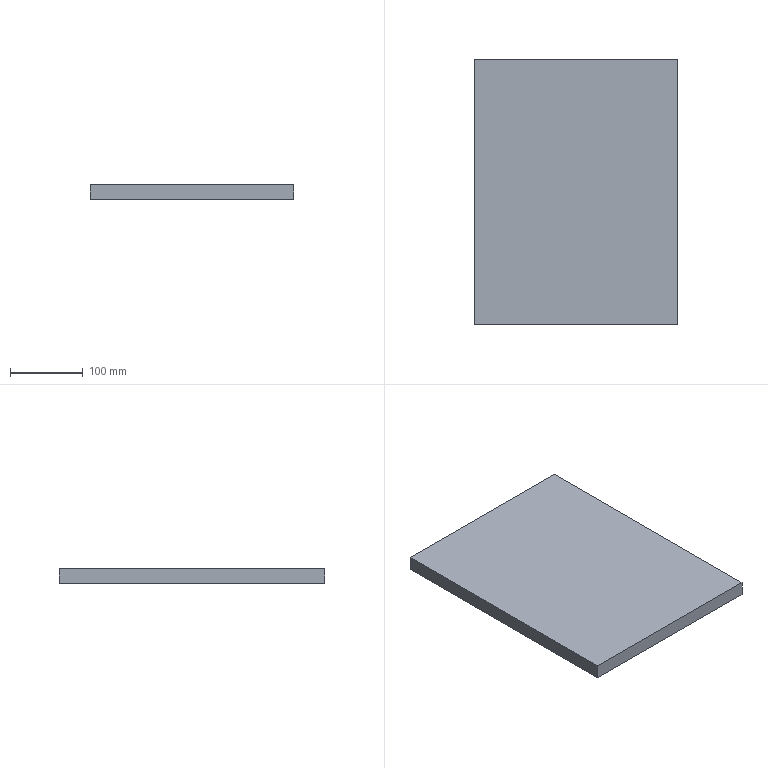Part | SolidWorks | features Extrusion 1 | 1 solid | 6 faces | box 280 x 365 x 20 mm | volume 2044000 mm3 | plane 6
STEP:
#1=CARTESIAN_POINT('',(0.,0.,0.));
#2=VERTEX_POINT('',#1);
#3=CARTESIAN_POINT('',(0.,365.,0.));
#4=VERTEX_POINT('',#3);
#5=CARTESIAN_POINT('',(0.,0.,0.));
#6=DIRECTION('',(0.,1.,0.));
#7=VECTOR('',#6,1000.);
#8=LINE('',#5,#7);
#9=EDGE_CURVE('',#2,#4,#8,.T.);
#10=ORIENTED_EDGE('',*,*,#9,.T.);
#11=CARTESIAN_POINT('',(0.,365.,20.));
#12=VERTEX_POINT('',#11);
#13=CARTESIAN_POINT('',(0.,365.,20.));
#14=DIRECTION('',(0.,0.,-1.));
#15=VECTOR('',#14,1000.);
#16=LINE('',#13,#15);
#17=EDGE_CURVE('',#12,#4,#16,.T.);
#18=ORIENTED_EDGE('',*,*,#17,.F.);
#19=CARTESIAN_POINT('',(0.,0.,20.));
#20=VERTEX_POINT('',#19);
#21=CARTESIAN_POINT('',(0.,0.,20.));
#22=DIRECTION('',(0.,1.,0.));
#23=VECTOR('',#22,1000.);
#24=LINE('',#21,#23);
#25=EDGE_CURVE('',#20,#12,#24,.T.);
#26=ORIENTED_EDGE('',*,*,#25,.F.);
#27=CARTESIAN_POINT('',(0.,0.,20.));
#28=DIRECTION('',(0.,0.,-1.));
#29=VECTOR('',#28,1000.);
#30=LINE('',#27,#29);
#31=EDGE_CURVE('',#20,#2,#30,.T.);
#32=ORIENTED_EDGE('',*,*,#31,.T.);
#33=EDGE_LOOP('',(#10,#18,#26,#32));
#34=FACE_OUTER_BOUND('',#33,.T.);
#35=CARTESIAN_POINT('',(0.,0.,20.));
#36=DIRECTION('',(-1.,0.,0.));
#37=DIRECTION('',(0.,0.,1.));
#38=AXIS2_PLACEMENT_3D('',#35,#36,#37);
#39=PLANE('',#38);
#40=ADVANCED_FACE('',(#34),#39,.F.);
#41=CARTESIAN_POINT('',(-280.,365.,0.));
#42=VERTEX_POINT('',#41);
#43=CARTESIAN_POINT('',(0.,365.,0.));
#44=DIRECTION('',(-1.,0.,0.));
#45=VECTOR('',#44,1000.);
#46=LINE('',#43,#45);
#47=EDGE_CURVE('',#4,#42,#46,.T.);
#48=ORIENTED_EDGE('',*,*,#47,.T.);
#49=CARTESIAN_POINT('',(-280.,365.,20.));
#50=VERTEX_POINT('',#49);
#51=CARTESIAN_POINT('',(-280.,365.,20.));
#52=DIRECTION('',(0.,0.,-1.));
#53=VECTOR('',#52,1000.);
#54=LINE('',#51,#53);
#55=EDGE_CURVE('',#50,#42,#54,.T.);
#56=ORIENTED_EDGE('',*,*,#55,.F.);
#57=CARTESIAN_POINT('',(0.,365.,20.));
#58=DIRECTION('',(-1.,0.,0.));
#59=VECTOR('',#58,1000.);
#60=LINE('',#57,#59);
#61=EDGE_CURVE('',#12,#50,#60,.T.);
#62=ORIENTED_EDGE('',*,*,#61,.F.);
#63=ORIENTED_EDGE('',*,*,#17,.T.);
#64=EDGE_LOOP('',(#48,#56,#62,#63));
#65=FACE_OUTER_BOUND('',#64,.T.);
#66=CARTESIAN_POINT('',(0.,365.,20.));
#67=DIRECTION('',(0.,-1.,0.));
#68=DIRECTION('',(1.,0.,0.));
#69=AXIS2_PLACEMENT_3D('',#66,#67,#68);
#70=PLANE('',#69);
#71=ADVANCED_FACE('',(#65),#70,.F.);
#72=CARTESIAN_POINT('',(-280.,0.,0.));
#73=VERTEX_POINT('',#72);
#74=CARTESIAN_POINT('',(-280.,0.,0.));
#75=DIRECTION('',(0.,-1.,0.));
#76=VECTOR('',#75,1000.);
#77=LINE('',#74,#76);
#78=EDGE_CURVE('',#42,#73,#77,.T.);
#79=ORIENTED_EDGE('',*,*,#78,.T.);
#80=CARTESIAN_POINT('',(-280.,0.,20.));
#81=VERTEX_POINT('',#80);
#82=CARTESIAN_POINT('',(-280.,0.,20.));
#83=DIRECTION('',(0.,0.,-1.));
#84=VECTOR('',#83,1000.);
#85=LINE('',#82,#84);
#86=EDGE_CURVE('',#81,#73,#85,.T.);
#87=ORIENTED_EDGE('',*,*,#86,.F.);
#88=CARTESIAN_POINT('',(-280.,0.,20.));
#89=DIRECTION('',(0.,-1.,0.));
#90=VECTOR('',#89,1000.);
#91=LINE('',#88,#90);
#92=EDGE_CURVE('',#50,#81,#91,.T.);
#93=ORIENTED_EDGE('',*,*,#92,.F.);
#94=ORIENTED_EDGE('',*,*,#55,.T.);
#95=EDGE_LOOP('',(#79,#87,#93,#94));
#96=FACE_OUTER_BOUND('',#95,.T.);
#97=CARTESIAN_POINT('',(-280.,0.,20.));
#98=DIRECTION('',(1.,0.,0.));
#99=DIRECTION('',(0.,0.,-1.));
#100=AXIS2_PLACEMENT_3D('',#97,#98,#99);
#101=PLANE('',#100);
#102=ADVANCED_FACE('',(#96),#101,.F.);
#103=CARTESIAN_POINT('',(0.,0.,0.));
#104=DIRECTION('',(1.,0.,0.));
#105=VECTOR('',#104,1000.);
#106=LINE('',#103,#105);
#107=EDGE_CURVE('',#73,#2,#106,.T.);
#108=ORIENTED_EDGE('',*,*,#107,.T.);
#109=ORIENTED_EDGE('',*,*,#31,.F.);
#110=CARTESIAN_POINT('',(0.,0.,20.));
#111=DIRECTION('',(1.,0.,0.));
#112=VECTOR('',#111,1000.);
#113=LINE('',#110,#112);
#114=EDGE_CURVE('',#81,#20,#113,.T.);
#115=ORIENTED_EDGE('',*,*,#114,.F.);
#116=ORIENTED_EDGE('',*,*,#86,.T.);
#117=EDGE_LOOP('',(#108,#109,#115,#116));
#118=FACE_OUTER_BOUND('',#117,.T.);
#119=CARTESIAN_POINT('',(0.,0.,20.));
#120=DIRECTION('',(0.,1.,0.));
#121=DIRECTION('',(-1.,0.,0.));
#122=AXIS2_PLACEMENT_3D('',#119,#120,#121);
#123=PLANE('',#122);
#124=ADVANCED_FACE('',(#118),#123,.F.);
#125=ORIENTED_EDGE('',*,*,#25,.T.);
#126=ORIENTED_EDGE('',*,*,#61,.T.);
#127=ORIENTED_EDGE('',*,*,#92,.T.);
#128=ORIENTED_EDGE('',*,*,#114,.T.);
#129=EDGE_LOOP('',(#125,#126,#127,#128));
#130=FACE_OUTER_BOUND('',#129,.T.);
#131=CARTESIAN_POINT('',(0.,0.,20.));
#132=DIRECTION('',(0.,0.,1.));
#133=DIRECTION('',(1.,0.,0.));
#134=AXIS2_PLACEMENT_3D('',#131,#132,#133);
#135=PLANE('',#134);
#136=ADVANCED_FACE('',(#130),#135,.T.);
#137=ORIENTED_EDGE('',*,*,#9,.F.);
#138=ORIENTED_EDGE('',*,*,#107,.F.);
#139=ORIENTED_EDGE('',*,*,#78,.F.);
#140=ORIENTED_EDGE('',*,*,#47,.F.);
#141=EDGE_LOOP('',(#137,#138,#139,#140));
#142=FACE_OUTER_BOUND('',#141,.T.);
#143=CARTESIAN_POINT('',(0.,0.,0.));
#144=DIRECTION('',(0.,0.,1.));
#145=DIRECTION('',(1.,0.,0.));
#146=AXIS2_PLACEMENT_3D('',#143,#144,#145);
#147=PLANE('',#146);
#148=ADVANCED_FACE('',(#142),#147,.F.);
#149=CLOSED_SHELL('',(#40,#71,#102,#124,#136,#148));
#150=MANIFOLD_SOLID_BREP('',#149);
#151=CARTESIAN_POINT('',(0.,0.,0.));
#152=DIRECTION('',(0.,0.,1.));
#153=DIRECTION('',(1.,0.,0.));
#154=AXIS2_PLACEMENT_3D('',#151,#152,#153);
#155=(LENGTH_UNIT()NAMED_UNIT(*)SI_UNIT(.MILLI.,.METRE.));
#156=UNCERTAINTY_MEASURE_WITH_UNIT(LENGTH_MEASURE(0.00001),#155,'','');
#157=(NAMED_UNIT(*)PLANE_ANGLE_UNIT()SI_UNIT($,.RADIAN.));
#158=(NAMED_UNIT(*)SI_UNIT($,.STERADIAN.)SOLID_ANGLE_UNIT());
#159=(GEOMETRIC_REPRESENTATION_CONTEXT(3)GLOBAL_UNCERTAINTY_ASSIGNED_CONTEXT((#156))GLOBAL_UNIT_ASSIGNED_CONTEXT((#155,#157,#158))REPRESENTATION_CONTEXT('',''));
#160=ADVANCED_BREP_SHAPE_REPRESENTATION('',(#150,#154),#159);